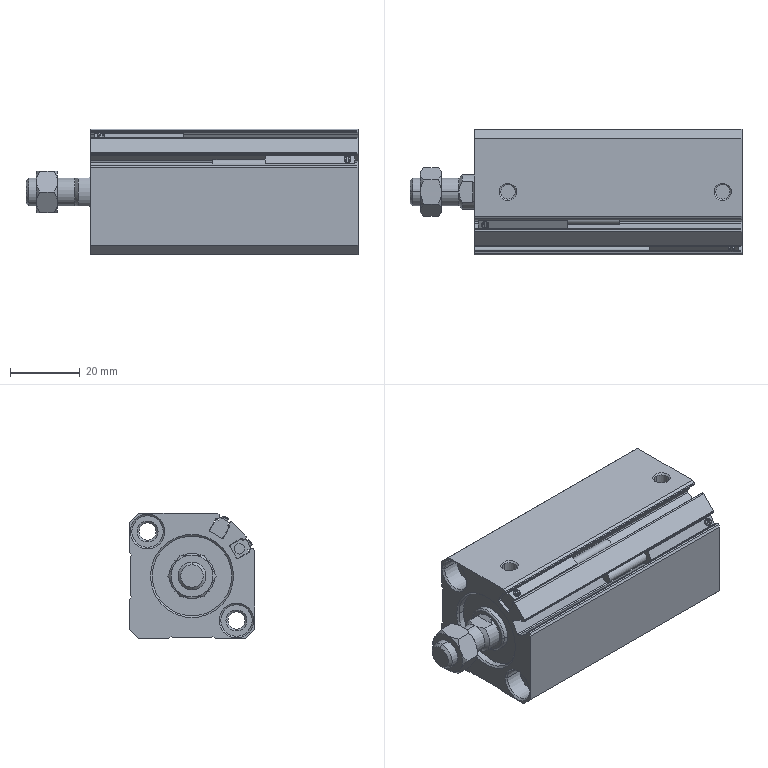Part | SolidWorks | 5 solids | 236 faces | box 95 x 36 x 36 mm | volume 77347 mm3 | plane 96 | cylinder 78 | cone 60 | torus 2 | commonest cylinder face diameters 0.8 x14 0.4 x10 9 x8 0.6 x4 1 x4 2 x4